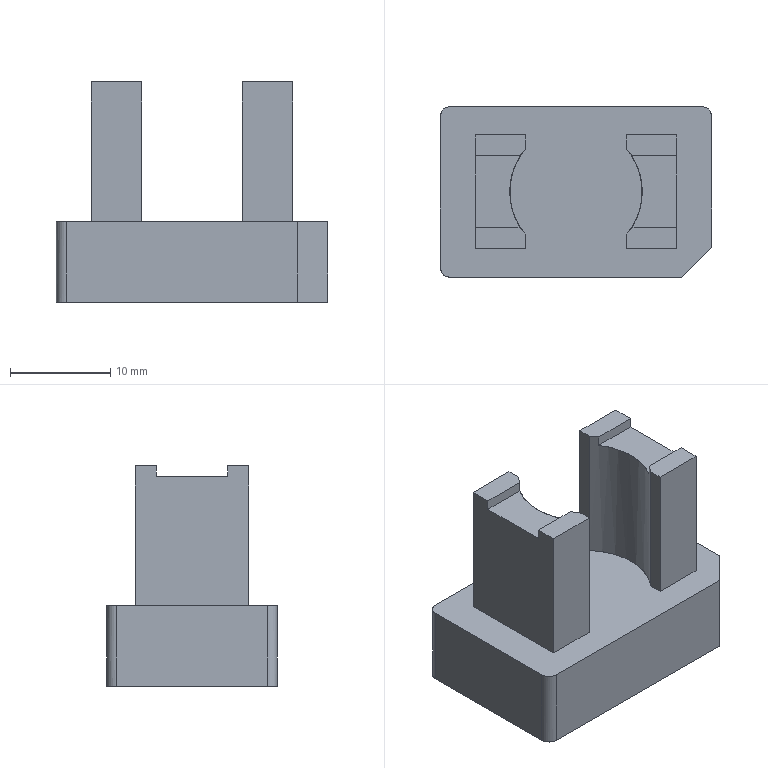NC program | PowerMill | posted with a generic post | part box 27 x 17 x 21.929 mm
Lines 16511 to 17293 of 116051:
N16608 M6
N16609 S18000 M03
N16610 G00 G90 X0.0 Y0.0
N16611 G43 Z10.799 H14
N16612
N16613 G05 P10000 R8
N16614 X11.0195 Y-8.1246
N16615 Z0.8798
N16616 G01 Z-0.3202 F1200.0
N16617 X11.0118 Y-8.0746 F2000.0
N16618 X11.0001 Y-8.0255
N16619 X10.9846 Y-7.9774
N16620 X10.9654 Y-7.9307
N16621 X10.9425 Y-7.8856
N16622 X10.9162 Y-7.8424
N16623 X10.8865 Y-7.8015
N16624 X10.8537 Y-7.7631
N16625 X10.818 Y-7.7274
N16626 X10.7795 Y-7.6946
N16627 X10.7386 Y-7.6649
N16628 X10.6955 Y-7.6386
N16629 X10.6505 Y-7.6157
N16630 X10.6037 Y-7.5965
N16631 X10.5556 Y-7.581
N16632 X10.5064 Y-7.5693
N16633 X10.4565 Y-7.5616
N16634 X10.4061 Y-7.5578
N16635 X10.3556 Y-7.5581
N16636 X10.3108 Y-7.5616
N16637 X10.2244 Y-7.5715
N16638 X10.1368 Y-7.5775
N16639 X10.0478 Y-7.5797
N16640 X9.9578
N16641 X6.4154 Y-7.5795
N16642 X4.9642 Y-7.5788
N16643 X4.8804 Y-7.5768
N16644 X4.7963 Y-7.5707
N16645 X4.7118 Y-7.5606
N16646 X4.6272 Y-7.5465
N16647 X4.5427 Y-7.5283
N16648 X4.4584 Y-7.5061
N16649 X4.3745 Y-7.48
N16650 X4.2913 Y-7.4498
N16651 X4.2102 Y-7.4163
N16652 X4.1308 Y-7.3791
N16653 X4.0532 Y-7.3383
N16654 X3.9776 Y-7.2941
N16655 X3.904 Y-7.2465
N16656 X3.8326 Y-7.1955
N16657 X3.7635 Y-7.1413
N16658 X3.6971 Y-7.0841
N16659 X3.6332 Y-7.0238
N16660 X3.5722 Y-6.9607
N16661 X3.514 Y-6.8948
N16662 X3.4607 Y-6.8288
N16663 X3.4105 Y-6.7605
N16664 X3.3628 Y-6.6888
N16665 X3.3175 Y-6.6137
N16666 X3.2748 Y-6.5351
N16667 X3.2348 Y-6.4531
N16668 X3.2066 Y-6.3895
N16669 X3.1811 Y-6.3248
N16670 X3.1583 Y-6.259
N16671 X3.1364 Y-6.1874
N16672 X3.1152 Y-6.1073
N16673 X3.096 Y-6.0207
N16674 X3.0812 Y-5.9365
N16675 X3.071 Y-5.8582
N16676 X3.0649 Y-5.7862
N16677 X3.0626 Y-5.7168
N16678 X3.0622 Y-5.6473
N16679 X3.0615 Y-5.1758
N16680 X3.0614 Y-4.3292
N16681 X3.0634 Y-4.2415
N16682 X3.0694 Y-4.154
N16683 X3.0794 Y-4.0669
N16684 X3.0933 Y-3.9805
N16685 X3.1112 Y-3.8949
N16686 X3.1329 Y-3.8103
N16687 X3.1584 Y-3.7269
N16688 X3.1877 Y-3.6448
N16689 X3.2206 Y-3.5641
N16690 X3.2576 Y-3.4836
N16691 X3.2977 Y-3.4057
N16692 X3.3408 Y-3.3307
N16693 X3.3867 Y-3.2586
N16694 X3.4354 Y-3.1895
N16695 X3.4868 Y-3.1229
N16696 X3.5434 Y-3.0539
N16697 X3.6013 Y-2.986
N16698 X3.6578 Y-2.9169
N16699 X3.694 Y-2.8708
N16700 X3.7288 Y-2.8256
N16701 X3.7618 Y-2.7819
N16702 X3.7928 Y-2.7397
N16703 X3.8232 Y-2.6974
N16704 X3.8532 Y-2.6548
N16705 X3.8826 Y-2.6118
N16706 X3.9115 Y-2.5685
N16707 X3.9401 Y-2.5249
N16708 X3.9684 Y-2.4812
N16709 X3.9971 Y-2.4377
N16710 X4.0271 Y-2.3951
N16711 X4.0591 Y-2.3541
N16712 X4.1127 Y-2.2898
N16713 X4.1688 Y-2.2277
N16714 X4.2274 Y-2.1681
N16715 X4.2896 Y-2.1102
N16716 X4.3561 Y-2.0537
N16717 X4.4242 Y-2.0007
N16718 X4.4929 Y-1.9514
N16719 X4.5554 Y-1.9103
N16720 X4.6231 Y-1.8703
N16721 X4.6979 Y-1.8306
N16722 X4.7813 Y-1.7907
N16723 X4.8577 Y-1.7579
N16724 X4.9371 Y-1.7282
N16725 X5.0195 Y-1.7016
N16726 X5.1049 Y-1.6782
N16727 X5.1859 Y-1.6598
N16728 X5.2705 Y-1.6445
N16729 X5.3507 Y-1.633
N16730 X5.395 Y-1.6281
N16731 X5.4395 Y-1.6258
N16732 X5.5053 Y-1.622
N16733 X5.5526 Y-1.621
N16734 X6.0284 Y-1.6208
N16735 X10.0437 Y-1.6206
N16736 X10.1322 Y-1.6226
N16737 X10.2203 Y-1.6286
N16738 X10.3077 Y-1.6385
N16739 X10.3943 Y-1.6523
N16740 X10.4799 Y-1.67
N16741 X10.5646 Y-1.6915
N16742 X10.6485 Y-1.717
N16743 X10.7311 Y-1.7463
N16744 X10.8124 Y-1.7793
N16745 X10.892 Y-1.8159
N16746 X10.9699 Y-1.8562
N16747 X11.046 Y-1.9
N16748 X11.1199 Y-1.9472
N16749 X11.1916 Y-1.9977
N16750 X11.2609 Y-2.0514
N16751 X11.3277 Y-2.1082
N16752 X11.3919 Y-2.168
N16753 X11.4532 Y-2.2307
N16754 X11.5117 Y-2.2961
N16755 X11.567 Y-2.3639
N16756 X11.6194 Y-2.4345
N16757 X11.6683 Y-2.507
N16758 X11.7135 Y-2.5813
N16759 X11.7552 Y-2.6572
N16760 X11.7931 Y-2.7345
N16761 X11.8272 Y-2.8131
N16762 X11.8578 Y-2.8931
N16763 X11.8864 Y-2.9775
N16764 X11.9101 Y-3.0591
N16765 X11.9293 Y-3.1384
N16766 X11.9426 Y-3.2069
N16767 X11.9535 Y-3.2757
N16768 X11.9617 Y-3.3448
N16769 X11.9674 Y-3.4142
N16770 X11.9712 Y-3.4966
N16771 X11.9726 Y-3.586
N16772 Y-3.6602
N16773 X11.9724 Y-3.7301
N16774 X11.9723 Y-3.7998
N16775 X11.9721 Y-4.9064
N16776 X11.9715 Y-5.7145
N16777 X11.9695 Y-5.7834
N16778 X11.9635 Y-5.8568
N16779 X11.9532 Y-5.9349
N16780 X11.9385 Y-6.017
N16781 X11.9199 Y-6.1003
N16782 X11.8969 Y-6.1877
N16783 X11.8711 Y-6.2709
N16784 X11.8419 Y-6.3519
N16785 X11.8089 Y-6.4317
N16786 X11.772 Y-6.5103
N16787 X11.7314 Y-6.5876
N16788 X11.6872 Y-6.6632
N16789 X11.6393 Y-6.7371
N16790 X11.588 Y-6.809
N16791 X11.5352 Y-6.8763
N16792 X11.4793 Y-6.9414
N16793 X11.4194 Y-7.0051
N16794 X11.3565 Y-7.0661
N16795 X11.2909 Y-7.1242
N16796 X11.2227 Y-7.1793
N16797 X11.1521 Y-7.2312
N16798 X11.0792 Y-7.2799
N16799 X11.0042 Y-7.3252
N16800 X10.9271 Y-7.367
N16801 X10.8482 Y-7.4053
N16802 X10.7676 Y-7.44
N16803 X10.6856 Y-7.4709
N16804 X10.6023 Y-7.4981
N16805 X10.5179 Y-7.5214
N16806 X10.4324 Y-7.5408
N16807 X10.3462 Y-7.5564
N16808 X10.3108 Y-7.5616
N16809 X10.2224 Y-7.5716 Z-0.3204
N16810 X10.1336 Y-7.5777 Z-0.3207
N16811 X10.0446 Y-7.5797 Z-0.3209
N16812 X9.9556 Z-0.3211
N16813 X7.2011 Y-7.5795 Z-0.3285
N16814 X4.9641 Y-7.5788 Z-0.3345
N16815 X4.8806 Y-7.5768 Z-0.3348
N16816 X4.7967 Y-7.5708 Z-0.335
N16817 X4.7125 Y-7.5607 Z-0.3352
N16818 X4.6282 Y-7.5467 Z-0.3354
N16819 X4.5439 Y-7.5286 Z-0.3357
N16820 X4.4597 Y-7.5064 Z-0.3359
N16821 X4.3759 Y-7.4802 Z-0.3361
N16822 X4.2926 Y-7.4501 Z-0.3364
N16823 X4.2101 Y-7.4159 Z-0.3366
N16824 X4.1315 Y-7.3793 Z-0.3368
N16825 X4.0545 Y-7.3391 Z-0.3371
N16826 X3.9794 Y-7.2954 Z-0.3373
N16827 X3.9061 Y-7.2481 Z-0.3376
N16828 X3.8349 Y-7.1975 Z-0.3378
N16829 X3.766 Y-7.1435 Z-0.338
N16830 X3.6995 Y-7.0863 Z-0.3383
N16831 X3.6355 Y-7.0261 Z-0.3385
N16832 X3.5745 Y-6.9632 Z-0.3387
N16833 X3.5164 Y-6.8975 Z-0.339
N16834 X3.4613 Y-6.8293 Z-0.3392
N16835 X3.4094 Y-6.7586 Z-0.3394
N16836 X3.3607 Y-6.6856 Z-0.3397
N16837 X3.3154 Y-6.6104 Z-0.3399
N16838 X3.2736 Y-6.5333 Z-0.3402
N16839 X3.2354 Y-6.4544 Z-0.3404
N16840 X3.2008 Y-6.3739 Z-0.3406
N16841 X3.1698 Y-6.2917 Z-0.3409
N16842 X3.1426 Y-6.2085 Z-0.3411
N16843 X3.1194 Y-6.1244 Z-0.3413
N16844 X3.1001 Y-6.0396 Z-0.3416
N16845 X3.0848 Y-5.9544 Z-0.3418
N16846 X3.0734 Y-5.8689 Z-0.342
N16847 X3.0661 Y-5.7833 Z-0.3422
N16848 X3.0627 Y-5.6975 Z-0.3425
N16849 X3.0606 Y-5.5312 Z-0.3429
N16850 X3.061 Y-5.3079 Z-0.3435
N16851 X3.0614 Y-5.0438 Z-0.3442
N16852 Y-4.3292 Z-0.3462
N16853 X3.0634 Y-4.2415 Z-0.3464
N16854 X3.0694 Y-4.1541 Z-0.3466
N16855 X3.0794 Y-4.067 Z-0.3469
N16856 X3.0934 Y-3.9805 Z-0.3471
N16857 X3.1113 Y-3.8946 Z-0.3473
N16858 X3.133 Y-3.8097 Z-0.3476
N16859 X3.1587 Y-3.7258 Z-0.3478
N16860 X3.1881 Y-3.6432 Z-0.348
N16861 X3.2212 Y-3.562 Z-0.3483
N16862 X3.2578 Y-3.4825 Z-0.3485
N16863 X3.2977 Y-3.4056 Z-0.3487
N16864 X3.3405 Y-3.3312 Z-0.349
N16865 X3.3864 Y-3.2597 Z-0.3492
N16866 X3.4351 Y-3.191 Z-0.3494
N16867 X3.4866 Y-3.1249 Z-0.3497
N16868 X3.5657 Y-3.0289 Z-0.35
N16869 X3.6252 Y-2.9574 Z-0.3502
N16870 X3.6919 Y-2.8745 Z-0.3505
N16871 X3.7368 Y-2.8152 Z-0.3507
N16872 X3.7811 Y-2.7554 Z-0.3509
N16873 X3.8246 Y-2.695 Z-0.3511
N16874 X3.888 Y-2.6014 Z-0.3514
N16875 X3.9681 Y-2.4804 Z-0.3518
N16876 X4.0154 Y-2.4129 Z-0.352
N16877 X4.0654 Y-2.3474 Z-0.3523
N16878 X4.1113 Y-2.2913 Z-0.3525
N16879 X4.1594 Y-2.2373 Z-0.3526
N16880 X4.21 Y-2.1848 Z-0.3528
N16881 X4.2735 Y-2.1241 Z-0.3531
N16882 X4.3396 Y-2.0665 Z-0.3533
N16883 X4.4083 Y-2.0119 Z-0.3536
N16884 X4.4793 Y-1.9605 Z-0.3538
N16885 X4.5526 Y-1.9124 Z-0.354
N16886 X4.6281 Y-1.8678 Z-0.3543
N16887 X4.7055 Y-1.8265 Z-0.3545
N16888 X4.7847 Y-1.7888 Z-0.3547
N16889 X4.8656 Y-1.7548 Z-0.355
N16890 X4.9479 Y-1.7245 Z-0.3552
N16891 X5.0316 Y-1.698 Z-0.3554
N16892 X5.1163 Y-1.6753 Z-0.3557
N16893 X5.2019 Y-1.6566 Z-0.3559
N16894 X5.2883 Y-1.6417 Z-0.3561
N16895 X5.3752 Y-1.6306 Z-0.3564
N16896 X5.4546 Y-1.6238 Z-0.3566
N16897 X5.5273 Y-1.6211 Z-0.3568
N16898 X5.5988 Y-1.621 Z-0.357
N16899 X6.9697 Y-1.6208 Z-0.3607
N16900 X9.9665 Y-1.6206 Z-0.3687
N16901 X10.0546 Z-0.3689
N16902 X10.1426 Y-1.623 Z-0.3692
N16903 X10.2304 Y-1.6295 Z-0.3694
N16904 X10.3178 Y-1.6399 Z-0.3697
N16905 X10.4046 Y-1.6542 Z-0.3699
N16906 X10.4906 Y-1.6725 Z-0.3701
N16907 X10.5755 Y-1.6947 Z-0.3704
N16908 X10.6593 Y-1.7206 Z-0.3706
N16909 X10.7416 Y-1.7503 Z-0.3708
N16910 X10.8226 Y-1.7837 Z-0.3711
N16911 X10.9019 Y-1.8208 Z-0.3713
N16912 X10.9796 Y-1.8615 Z-0.3715
N16913 X11.0554 Y-1.9057 Z-0.3718
N16914 X11.1291 Y-1.9534 Z-0.372
N16915 X11.2005 Y-2.0043 Z-0.3723
N16916 X11.2696 Y-2.0584 Z-0.3725
N16917 X11.3361 Y-2.1157 Z-0.3727
N16918 X11.3999 Y-2.1759 Z-0.373
N16919 X11.4609 Y-2.2389 Z-0.3732
N16920 X11.5191 Y-2.3047 Z-0.3734
N16921 X11.574 Y-2.3728 Z-0.3737
N16922 X11.6254 Y-2.4429 Z-0.3739
N16923 X11.6733 Y-2.5149 Z-0.3741
N16924 X11.7176 Y-2.5886 Z-0.3744
N16925 X11.7582 Y-2.6639 Z-0.3746
N16926 X11.7952 Y-2.7407 Z-0.3748
N16927 X11.8317 Y-2.8249 Z-0.3751
N16928 X11.8627 Y-2.9053 Z-0.3753
N16929 X11.8886 Y-2.9828 Z-0.3755
N16930 X11.9098 Y-3.0583 Z-0.3757
N16931 X11.9255 Y-3.1236 Z-0.3759
N16932 X11.939 Y-3.1894 Z-0.3761
N16933 X11.9503 Y-3.2554 Z-0.3763
N16934 X11.9591 Y-3.3219 Z-0.3764
N16935 X11.9657 Y-3.3924 Z-0.3766
N16936 X11.9703 Y-3.4763 Z-0.3769
N16937 X11.9722 Y-3.5615 Z-0.3771
N16938 X11.9725 Y-3.6349 Z-0.3773
N16939 X11.9724 Y-3.7023 Z-0.3775
N16940 X11.9723 Y-3.7696 Z-0.3776
N16941 X11.9724 Y-4.9064 Z-0.3807
N16942 X11.9725 Y-5.3682 Z-0.3819
N16943 X11.9722 Y-5.6203 Z-0.3826
N16944 X11.9716 Y-5.7145 Z-0.3829
N16945 X11.969 Y-5.7868 Z-0.3831
N16946 X11.9623 Y-5.8631 Z-0.3833
N16947 X11.9515 Y-5.9437 Z-0.3835
N16948 X11.9362 Y-6.0276 Z-0.3837
N16949 X11.9169 Y-6.1131 Z-0.384
N16950 X11.8935 Y-6.1997 Z-0.3842
N16951 X11.8668 Y-6.2833 Z-0.3844
N16952 X11.837 Y-6.364 Z-0.3847
N16953 X11.8036 Y-6.4432 Z-0.3849
N16954 X11.7659 Y-6.5223 Z-0.3851
N16955 X11.7246 Y-6.5997 Z-0.3854
N16956 X11.6798 Y-6.6751 Z-0.3856
N16957 X11.6316 Y-6.7484 Z-0.3858
N16958 X11.5801 Y-6.8195 Z-0.3861
N16959 X11.5255 Y-6.8881 Z-0.3863
N16960 X11.4678 Y-6.9541 Z-0.3865
N16961 X11.4071 Y-7.0174 Z-0.3868
N16962 X11.3436 Y-7.0779 Z-0.387
N16963 X11.2775 Y-7.1355 Z-0.3872
N16964 X11.2088 Y-7.19 Z-0.3875
N16965 X11.1377 Y-7.2413 Z-0.3877
N16966 X11.0643 Y-7.2893 Z-0.3879
N16967 X10.9888 Y-7.3339 Z-0.3882
N16968 X10.9113 Y-7.375 Z-0.3884
N16969 X10.832 Y-7.4126 Z-0.3887
N16970 X10.7511 Y-7.4465 Z-0.3889
N16971 X10.6688 Y-7.4767 Z-0.3891
N16972 X10.5852 Y-7.5031 Z-0.3894
N16973 X10.5004 Y-7.5256 Z-0.3896
N16974 X10.4148 Y-7.5443 Z-0.3898
N16975 X10.3283 Y-7.5591 Z-0.3901
N16976 X10.3108 Y-7.5616
N16977 X10.2224 Y-7.5716 Z-0.3904
N16978 X10.1336 Y-7.5777 Z-0.3906
N16979 X10.0446 Y-7.5797 Z-0.3908
N16980 X9.9556 Z-0.3911
N16981 X7.2011 Y-7.5795 Z-0.3985
N16982 X4.9641 Y-7.5788 Z-0.4045
N16983 X4.8806 Y-7.5768 Z-0.4047
N16984 X4.7967 Y-7.5708 Z-0.4049
N16985 X4.7125 Y-7.5607 Z-0.4052
N16986 X4.6282 Y-7.5467 Z-0.4054
N16987 X4.5439 Y-7.5286 Z-0.4056
N16988 X4.4597 Y-7.5064 Z-0.4059
N16989 X4.3759 Y-7.4802 Z-0.4061
N16990 X4.2926 Y-7.4501 Z-0.4063
N16991 X4.2101 Y-7.4159 Z-0.4066
N16992 X4.1315 Y-7.3793 Z-0.4068
N16993 X4.0545 Y-7.3391 Z-0.407
N16994 X3.9794 Y-7.2954 Z-0.4073
N16995 X3.9061 Y-7.2481 Z-0.4075
N16996 X3.8349 Y-7.1975 Z-0.4077
N16997 X3.766 Y-7.1435 Z-0.408
N16998 X3.6995 Y-7.0863 Z-0.4082
N16999 X3.6355 Y-7.0261 Z-0.4085
N17000 X3.5745 Y-6.9632 Z-0.4087
N17001 X3.5164 Y-6.8975 Z-0.4089
N17002 X3.4613 Y-6.8293 Z-0.4091
N17003 X3.4094 Y-6.7586 Z-0.4094
N17004 X3.3607 Y-6.6856 Z-0.4096
N17005 X3.3154 Y-6.6104 Z-0.4099
N17006 X3.2736 Y-6.5333 Z-0.4101
N17007 X3.2354 Y-6.4544 Z-0.4103
N17008 X3.2008 Y-6.3739 Z-0.4106
N17009 X3.1698 Y-6.2917 Z-0.4108
N17010 X3.1426 Y-6.2085 Z-0.411
N17011 X3.1194 Y-6.1244 Z-0.4113
N17012 X3.1001 Y-6.0396 Z-0.4115
N17013 X3.0848 Y-5.9544 Z-0.4117
N17014 X3.0734 Y-5.8689 Z-0.412
N17015 X3.0661 Y-5.7833 Z-0.4122
N17016 X3.0627 Y-5.6975 Z-0.4124
N17017 X3.0606 Y-5.5312 Z-0.4129
N17018 X3.061 Y-5.3079 Z-0.4135
N17019 X3.0614 Y-5.0438 Z-0.4142
N17020 Y-4.3292 Z-0.4161
N17021 X3.0634 Y-4.2415 Z-0.4163
N17022 X3.0694 Y-4.1541 Z-0.4166
N17023 X3.0794 Y-4.067 Z-0.4168
N17024 X3.0934 Y-3.9805 Z-0.417
N17025 X3.1113 Y-3.8946 Z-0.4173
N17026 X3.133 Y-3.8097 Z-0.4175
N17027 X3.1587 Y-3.7258 Z-0.4178
N17028 X3.1881 Y-3.6432 Z-0.418
N17029 X3.2212 Y-3.562 Z-0.4182
N17030 X3.2578 Y-3.4825 Z-0.4185
N17031 X3.2977 Y-3.4056 Z-0.4187
N17032 X3.3405 Y-3.3312 Z-0.4189
N17033 X3.3864 Y-3.2597 Z-0.4192
N17034 X3.4351 Y-3.191 Z-0.4194
N17035 X3.4866 Y-3.1249 Z-0.4196
N17036 X3.5657 Y-3.0289 Z-0.4199
N17037 X3.6252 Y-2.9574 Z-0.4202
N17038 X3.6919 Y-2.8745 Z-0.4205
N17039 X3.7368 Y-2.8152 Z-0.4207
N17040 X3.7811 Y-2.7554 Z-0.4209
N17041 X3.8246 Y-2.695 Z-0.4211
N17042 X3.888 Y-2.6014 Z-0.4214
N17043 X3.9681 Y-2.4804 Z-0.4218
N17044 X4.0154 Y-2.4129 Z-0.422
N17045 X4.0654 Y-2.3474 Z-0.4222
N17046 X4.1113 Y-2.2913 Z-0.4224
N17047 X4.1594 Y-2.2372 Z-0.4226
N17048 X4.21 Y-2.1848 Z-0.4228
N17049 X4.2735 Y-2.1242 Z-0.423
N17050 X4.3396 Y-2.0665 Z-0.4233
N17051 X4.4082 Y-2.0119 Z-0.4235
N17052 X4.4793 Y-1.9605 Z-0.4237
N17053 X4.5526 Y-1.9125 Z-0.424
N17054 X4.628 Y-1.8678 Z-0.4242
N17055 X4.7055 Y-1.8265 Z-0.4244
N17056 X4.7847 Y-1.7889 Z-0.4247
N17057 X4.8656 Y-1.7548 Z-0.4249
N17058 X4.9479 Y-1.7245 Z-0.4251
N17059 X5.0316 Y-1.698 Z-0.4254
N17060 X5.1162 Y-1.6754 Z-0.4256
N17061 X5.2019 Y-1.6566 Z-0.4259
N17062 X5.2882 Y-1.6417 Z-0.4261
N17063 X5.3751 Y-1.6306 Z-0.4263
N17064 X5.4546 Y-1.6238 Z-0.4265
N17065 X5.5273 Y-1.6211 Z-0.4267
N17066 X5.5988 Y-1.621 Z-0.4269
N17067 X6.9701 Y-1.6208 Z-0.4306
N17068 X9.967 Y-1.6206 Z-0.4387
N17069 X10.0551 Z-0.4389
N17070 X10.1431 Y-1.6231 Z-0.4391
N17071 X10.2309 Y-1.6295 Z-0.4394
N17072 X10.3183 Y-1.6399 Z-0.4396
N17073 X10.4051 Y-1.6543 Z-0.4398
N17074 X10.491 Y-1.6726 Z-0.4401
N17075 X10.5759 Y-1.6948 Z-0.4403
N17076 X10.6597 Y-1.7207 Z-0.4405
N17077 X10.7421 Y-1.7505 Z-0.4408
N17078 X10.823 Y-1.7839 Z-0.441
N17079 X10.9023 Y-1.821 Z-0.4412
N17080 X10.98 Y-1.8617 Z-0.4415
N17081 X11.0558 Y-1.906 Z-0.4417
N17082 X11.1295 Y-1.9536 Z-0.442
N17083 X11.2009 Y-2.0046 Z-0.4422
N17084 X11.2699 Y-2.0587 Z-0.4424
N17085 X11.3364 Y-2.116 Z-0.4427
N17086 X11.4002 Y-2.1762 Z-0.4429
N17087 X11.4612 Y-2.2392 Z-0.4431
N17088 X11.5194 Y-2.3051 Z-0.4434
N17089 X11.5742 Y-2.3731 Z-0.4436
N17090 X11.6257 Y-2.4433 Z-0.4438
N17091 X11.6736 Y-2.5153 Z-0.4441
N17092 X11.7178 Y-2.589 Z-0.4443
N17093 X11.7584 Y-2.6643 Z-0.4445
N17094 X11.7954 Y-2.7411 Z-0.4448
N17095 X11.8319 Y-2.8252 Z-0.445
N17096 X11.8628 Y-2.9056 Z-0.4452
N17097 X11.8887 Y-2.9832 Z-0.4455
N17098 X11.9099 Y-3.0586 Z-0.4457
N17099 X11.9255 Y-3.124 Z-0.4459
N17100 X11.9391 Y-3.1897 Z-0.446
N17101 X11.9504 Y-3.2558 Z-0.4462
N17102 X11.9591 Y-3.3223 Z-0.4464
N17103 X11.9657 Y-3.3929 Z-0.4466
N17104 X11.9703 Y-3.4768 Z-0.4468
N17105 X11.9722 Y-3.562 Z-0.447
N17106 X11.9725 Y-3.6352 Z-0.4472
N17107 X11.9724 Y-3.7027 Z-0.4474
N17108 X11.9723 Y-3.77 Z-0.4476
N17109 X11.9724 Y-4.9064 Z-0.4506
N17110 X11.9725 Y-5.3682 Z-0.4519
N17111 X11.9722 Y-5.6203 Z-0.4526
N17112 X11.9716 Y-5.7145 Z-0.4528
N17113 X11.969 Y-5.7868 Z-0.453
N17114 X11.9623 Y-5.8631 Z-0.4532
N17115 X11.9515 Y-5.9437 Z-0.4534
N17116 X11.9362 Y-6.0276 Z-0.4537
N17117 X11.9169 Y-6.1131 Z-0.4539
N17118 X11.8935 Y-6.1997 Z-0.4541
N17119 X11.8668 Y-6.2833 Z-0.4544
N17120 X11.837 Y-6.364 Z-0.4546
N17121 X11.8036 Y-6.4432 Z-0.4548
N17122 X11.7659 Y-6.5223 Z-0.4551
N17123 X11.7246 Y-6.5997 Z-0.4553
N17124 X11.6798 Y-6.6751 Z-0.4556
N17125 X11.6316 Y-6.7484 Z-0.4558
N17126 X11.5801 Y-6.8195 Z-0.456
N17127 X11.5255 Y-6.8881 Z-0.4563
N17128 X11.4678 Y-6.9541 Z-0.4565
N17129 X11.4071 Y-7.0174 Z-0.4567
N17130 X11.3436 Y-7.0779 Z-0.457
N17131 X11.2775 Y-7.1355 Z-0.4572
N17132 X11.2088 Y-7.19 Z-0.4574
N17133 X11.1377 Y-7.2413 Z-0.4577
N17134 X11.0643 Y-7.2893 Z-0.4579
N17135 X10.9888 Y-7.3339 Z-0.4581
N17136 X10.9113 Y-7.375 Z-0.4584
N17137 X10.832 Y-7.4126 Z-0.4586
N17138 X10.7511 Y-7.4465 Z-0.4589
N17139 X10.6688 Y-7.4767 Z-0.4591
N17140 X10.5852 Y-7.5031 Z-0.4593
N17141 X10.5004 Y-7.5256 Z-0.4596
N17142 X10.4148 Y-7.5443 Z-0.4598
N17143 X10.3283 Y-7.5591 Z-0.46
N17144 X10.3108 Y-7.5616 Z-0.4601
N17145 X10.2224 Y-7.5716 Z-0.4603
N17146 X10.1336 Y-7.5777 Z-0.4605
N17147 X10.0446 Y-7.5797 Z-0.4608
N17148 X9.9556 Z-0.461
N17149 X7.2011 Y-7.5795 Z-0.4684
N17150 X4.9641 Y-7.5788 Z-0.4744
N17151 X4.8806 Y-7.5768 Z-0.4747
N17152 X4.7967 Y-7.5708 Z-0.4749
N17153 X4.7125 Y-7.5607 Z-0.4751
N17154 X4.6282 Y-7.5467 Z-0.4753
N17155 X4.5439 Y-7.5286 Z-0.4756
N17156 X4.4597 Y-7.5064 Z-0.4758
N17157 X4.3759 Y-7.4802 Z-0.476
N17158 X4.2926 Y-7.4501 Z-0.4763
N17159 X4.2101 Y-7.4159 Z-0.4765
N17160 X4.1315 Y-7.3793 Z-0.4767
N17161 X4.0545 Y-7.3391 Z-0.477
N17162 X3.9794 Y-7.2954 Z-0.4772
N17163 X3.9061 Y-7.2481 Z-0.4775
N17164 X3.8349 Y-7.1975 Z-0.4777
N17165 X3.766 Y-7.1435 Z-0.4779
N17166 X3.6995 Y-7.0863 Z-0.4782
N17167 X3.6355 Y-7.0261 Z-0.4784
N17168 X3.5745 Y-6.9632 Z-0.4786
N17169 X3.5164 Y-6.8975 Z-0.4789
N17170 X3.4613 Y-6.8293 Z-0.4791
N17171 X3.4094 Y-6.7586 Z-0.4793
N17172 X3.3607 Y-6.6856 Z-0.4796
N17173 X3.3154 Y-6.6104 Z-0.4798
N17174 X3.2736 Y-6.5333 Z-0.48
N17175 X3.2354 Y-6.4544 Z-0.4803
N17176 X3.2008 Y-6.3739 Z-0.4805
N17177 X3.1698 Y-6.2917 Z-0.4808
N17178 X3.1426 Y-6.2085 Z-0.481
N17179 X3.1194 Y-6.1244 Z-0.4812
N17180 X3.1001 Y-6.0396 Z-0.4815
N17181 X3.0848 Y-5.9544 Z-0.4817
N17182 X3.0734 Y-5.8689 Z-0.4819
N17183 X3.0661 Y-5.7833 Z-0.4821
N17184 X3.0627 Y-5.6975 Z-0.4824
N17185 X3.0606 Y-5.5312 Z-0.4828
N17186 X3.061 Y-5.3079 Z-0.4834
N17187 X3.0614 Y-5.0438 Z-0.4841
N17188 Y-4.3292 Z-0.4861
N17189 X3.0634 Y-4.2415 Z-0.4863
N17190 X3.0694 Y-4.1541 Z-0.4865
N17191 X3.0794 Y-4.067 Z-0.4868
N17192 X3.0934 Y-3.9805 Z-0.487
N17193 X3.1113 Y-3.8946 Z-0.4872
N17194 X3.133 Y-3.8097 Z-0.4875
N17195 X3.1587 Y-3.7258 Z-0.4877
N17196 X3.1881 Y-3.6432 Z-0.4879
N17197 X3.2212 Y-3.562 Z-0.4882
N17198 X3.2578 Y-3.4825 Z-0.4884
N17199 X3.2977 Y-3.4056 Z-0.4886
N17200 X3.3405 Y-3.3312 Z-0.4889
N17201 X3.3864 Y-3.2597 Z-0.4891
N17202 X3.4351 Y-3.191 Z-0.4893
N17203 X3.4866 Y-3.1249 Z-0.4896
N17204 X3.5657 Y-3.0289 Z-0.4899
N17205 X3.6252 Y-2.9574 Z-0.4901
N17206 X3.6919 Y-2.8745 Z-0.4904
N17207 X3.7368 Y-2.8152 Z-0.4906
N17208 X3.7811 Y-2.7554 Z-0.4908
N17209 X3.8245 Y-2.695 Z-0.491
N17210 X3.8879 Y-2.6014 Z-0.4913
N17211 X3.9681 Y-2.4804 Z-0.4917
N17212 X4.0154 Y-2.4129 Z-0.4919
N17213 X4.0654 Y-2.3474 Z-0.4922
N17214 X4.1113 Y-2.2913 Z-0.4924
N17215 X4.1594 Y-2.2373 Z-0.4925
N17216 X4.21 Y-2.1848 Z-0.4927
N17217 X4.2735 Y-2.1241 Z-0.493
N17218 X4.3396 Y-2.0665 Z-0.4932
N17219 X4.4083 Y-2.0119 Z-0.4934
N17220 X4.4793 Y-1.9605 Z-0.4937
N17221 X4.5526 Y-1.9124 Z-0.4939
N17222 X4.6281 Y-1.8677 Z-0.4942
N17223 X4.7055 Y-1.8265 Z-0.4944
N17224 X4.7847 Y-1.7888 Z-0.4946
N17225 X4.8656 Y-1.7548 Z-0.4949
N17226 X4.948 Y-1.7245 Z-0.4951
N17227 X5.0316 Y-1.698 Z-0.4953
N17228 X5.1163 Y-1.6753 Z-0.4956
N17229 X5.2019 Y-1.6566 Z-0.4958
N17230 X5.2883 Y-1.6417 Z-0.496
N17231 X5.3752 Y-1.6306 Z-0.4963
N17232 X5.4546 Y-1.6238 Z-0.4965
N17233 X5.5273 Y-1.6211 Z-0.4967
N17234 X5.5988 Y-1.621 Z-0.4969
N17235 X7.0 Y-1.6208 Z-0.5006
N17236 X10.0437 Y-1.6205 Z-0.5088
N17237 X10.1315 Y-1.6225 Z-0.509
N17238 X10.2192 Y-1.6284 Z-0.5093
N17239 X10.3066 Y-1.6383 Z-0.5095
N17240 X10.3934 Y-1.6522 Z-0.5098
N17241 X10.4794 Y-1.67 Z-0.51
N17242 X10.5646 Y-1.6916 Z-0.5102
N17243 X10.6487 Y-1.7172 Z-0.5105
N17244 X10.7315 Y-1.7465 Z-0.5107
N17245 X10.8128 Y-1.7795 Z-0.5109
N17246 X10.8924 Y-1.8161 Z-0.5112
N17247 X10.9703 Y-1.8563 Z-0.5114
N17248 X11.0462 Y-1.9001 Z-0.5116
N17249 X11.1197 Y-1.947 Z-0.5119
N17250 X11.1912 Y-1.9973 Z-0.5121
N17251 X11.2605 Y-2.0511 Z-0.5123
N17252 X11.3275 Y-2.108 Z-0.5126
N17253 X11.3918 Y-2.168 Z-0.5128
N17254 X11.4532 Y-2.2307 Z-0.5131
N17255 X11.5117 Y-2.296 Z-0.5133
N17256 X11.5669 Y-2.3638 Z-0.5135
N17257 X11.6188 Y-2.4338 Z-0.5138
N17258 X11.6673 Y-2.5058 Z-0.514
N17259 X11.7134 Y-2.5812 Z-0.5142
N17260 X11.7558 Y-2.6585 Z-0.5145
N17261 X11.7945 Y-2.737 Z-0.5147
N17262 X11.8292 Y-2.8165 Z-0.5149
N17263 X11.8599 Y-2.8964 Z-0.5152
N17264 X11.8864 Y-2.9765 Z-0.5154
N17265 X11.9058 Y-3.0444 Z-0.5156
N17266 X11.923 Y-3.1129 Z-0.5158
N17267 X11.9376 Y-3.1818 Z-0.516
N17268 X11.9496 Y-3.2513 Z-0.5162
N17269 X11.9593 Y-3.3263 Z-0.5164
N17270 X11.9668 Y-3.411 Z-0.5166
N17271 X11.9713 Y-3.5009 Z-0.5168
N17272 X11.9731 Y-3.5824 Z-0.517
N17273 X11.9736 Y-3.6581 Z-0.5172
N17274 Y-3.7303 Z-0.5174
N17275 X11.9734 Y-3.8035 Z-0.5176
N17276 X11.9725 Y-4.7405 Z-0.5202
N17277 Y-5.3682 Z-0.5218
N17278 X11.9722 Y-5.6203 Z-0.5225
N17279 X11.9716 Y-5.7145 Z-0.5228
N17280 X11.969 Y-5.7868 Z-0.523
N17281 X11.9623 Y-5.8631 Z-0.5232
N17282 X11.9515 Y-5.9437 Z-0.5234
N17283 X11.9362 Y-6.0276 Z-0.5236
N17284 X11.9169 Y-6.1131 Z-0.5239
N17285 X11.8935 Y-6.1997 Z-0.5241
N17286 X11.8668 Y-6.2833 Z-0.5243
N17287 X11.837 Y-6.364 Z-0.5246
N17288 X11.8036 Y-6.4432 Z-0.5248
N17289 X11.7659 Y-6.5223 Z-0.525
N17290 X11.7246 Y-6.5997 Z-0.5253
N17291 X11.6798 Y-6.6751 Z-0.5255
N17292 X11.6316 Y-6.7484 Z-0.5257
N17293 X11.5801 Y-6.8195 Z-0.526
N17294 X11.5255 Y-6.8881 Z-0.5262
N17295 X11.4678 Y-6.9541 Z-0.5264
N17296 X11.4071 Y-7.0174 Z-0.5267
N17297 X11.3436 Y-7.0779 Z-0.5269
N17298 X11.2775 Y-7.1355 Z-0.5271
N17299 X11.2088 Y-7.19 Z-0.5274
N17300 X11.1377 Y-7.2413 Z-0.5276
N17301 X11.0643 Y-7.2893 Z-0.5278
N17302 X10.9888 Y-7.3339 Z-0.5281
N17303 X10.9113 Y-7.375 Z-0.5283
N17304 X10.832 Y-7.4126 Z-0.5286
N17305 X10.7511 Y-7.4465 Z-0.5288
N17306 X10.6688 Y-7.4767 Z-0.529
N17307 X10.5852 Y-7.5031 Z-0.5293
N17308 X10.5004 Y-7.5256 Z-0.5295
N17309 X10.4148 Y-7.5443 Z-0.5297
N17310 X10.3283 Y-7.5591 Z-0.53
N17311 X10.3108 Y-7.5616
N17312 X10.2224 Y-7.5716 Z-0.5303
N17313 X10.1336 Y-7.5777 Z-0.5305
N17314 X10.0446 Y-7.5797 Z-0.5307
N17315 X9.9556 Z-0.531
N17316 X7.2011 Y-7.5795 Z-0.5384
N17317 X4.9641 Y-7.5788 Z-0.5444
N17318 X4.8806 Y-7.5768 Z-0.5446
N17319 X4.7967 Y-7.5708 Z-0.5448
N17320 X4.7125 Y-7.5607 Z-0.5451
N17321 X4.6282 Y-7.5467 Z-0.5453
N17322 X4.5439 Y-7.5286 Z-0.5455
N17323 X4.4597 Y-7.5064 Z-0.5458
N17324 X4.3759 Y-7.4802 Z-0.546
N17325 X4.2926 Y-7.4501 Z-0.5462
N17326 X4.2101 Y-7.4159 Z-0.5465
N17327 X4.1315 Y-7.3793 Z-0.5467
N17328 X4.0545 Y-7.3391 Z-0.5469
N17329 X3.9794 Y-7.2954 Z-0.5472
N17330 X3.9061 Y-7.2481 Z-0.5474
N17331 X3.8349 Y-7.1975 Z-0.5476
N17332 X3.766 Y-7.1435 Z-0.5479
N17333 X3.6995 Y-7.0863 Z-0.5481
N17334 X3.6355 Y-7.0261 Z-0.5483
N17335 X3.5745 Y-6.9632 Z-0.5486
N17336 X3.5164 Y-6.8975 Z-0.5488
N17337 X3.4613 Y-6.8293 Z-0.549
N17338 X3.4094 Y-6.7586 Z-0.5493
N17339 X3.3607 Y-6.6856 Z-0.5495
N17340 X3.3154 Y-6.6104 Z-0.5498
N17341 X3.2736 Y-6.5333 Z-0.55
N17342 X3.2354 Y-6.4544 Z-0.5502
N17343 X3.2008 Y-6.3739 Z-0.5505
N17344 X3.1698 Y-6.2917 Z-0.5507
N17345 X3.1426 Y-6.2085 Z-0.5509
N17346 X3.1194 Y-6.1244 Z-0.5512
N17347 X3.1001 Y-6.0396 Z-0.5514
N17348 X3.0848 Y-5.9544 Z-0.5516
N17349 X3.0734 Y-5.8689 Z-0.5519
N17350 X3.0661 Y-5.7833 Z-0.5521
N17351 X3.0627 Y-5.6975 Z-0.5523
N17352 X3.0606 Y-5.5312 Z-0.5528
N17353 X3.061 Y-5.3079 Z-0.5534
N17354 X3.0614 Y-5.0438 Z-0.5541
N17355 Y-4.3292 Z-0.556
N17356 X3.0634 Y-4.2415 Z-0.5562
N17357 X3.0694 Y-4.1541 Z-0.5565
N17358 X3.0794 Y-4.067 Z-0.5567
N17359 X3.0934 Y-3.9805 Z-0.5569
N17360 X3.1113 Y-3.8946 Z-0.5572
N17361 X3.133 Y-3.8097 Z-0.5574
N17362 X3.1587 Y-3.7258 Z-0.5576
N17363 X3.1881 Y-3.6432 Z-0.5579
N17364 X3.2212 Y-3.562 Z-0.5581
N17365 X3.2578 Y-3.4825 Z-0.5584
N17366 X3.2977 Y-3.4055 Z-0.5586
N17367 X3.3406 Y-3.3312 Z-0.5588
N17368 X3.3864 Y-3.2597 Z-0.559
N17369 X3.4351 Y-3.191 Z-0.5593
N17370 X3.4866 Y-3.1249 Z-0.5595
N17371 X3.5656 Y-3.029 Z-0.5598
N17372 X3.625 Y-2.9575 Z-0.5601
N17373 X3.6917 Y-2.8747 Z-0.5604
N17374 X3.7365 Y-2.8156 Z-0.5606
N17375 X3.7807 Y-2.756 Z-0.5608
N17376 X3.824 Y-2.6958 Z-0.561
N17377 X3.8873 Y-2.6023 Z-0.5613
N17378 X3.9681 Y-2.4804 Z-0.5617
N17379 X4.0154 Y-2.4129 Z-0.5619
N17380 X4.0654 Y-2.3474 Z-0.5621
N17381 X4.1112 Y-2.2913 Z-0.5623
N17382 X4.1594 Y-2.2373 Z-0.5625
N17383 X4.21 Y-2.1848 Z-0.5627
N17384 X4.2735 Y-2.1241 Z-0.5629
N17385 X4.3396 Y-2.0665 Z-0.5632
N17386 X4.4082 Y-2.0119 Z-0.5634
N17387 X4.4793 Y-1.9605 Z-0.5636
N17388 X4.5526 Y-1.9125 Z-0.5639
N17389 X4.628 Y-1.8678 Z-0.5641
N17390 X4.7055 Y-1.8265 Z-0.5643